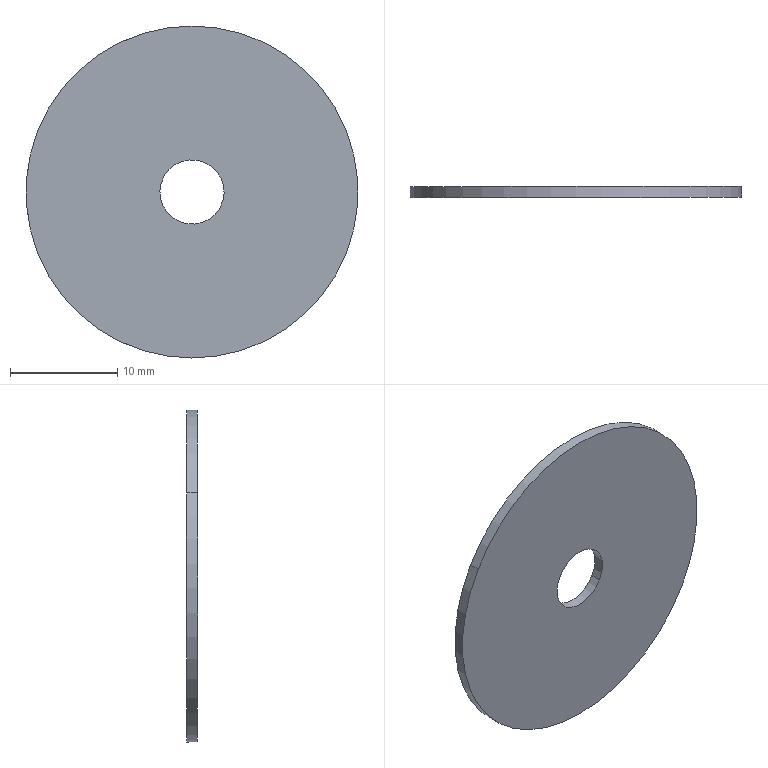Part | SolidWorks | features BaseBody 1 | 1 solid | 6 faces | box 31.001 x 1.03 x 31 mm | volume 726.493 mm3 | cylinder 4 | plane 2 | commonest cylinder face diameters 6 x2 31 x2
STEP:
#1=CARTESIAN_POINT('',(344.556,387.967,105.419));
#2=VERTEX_POINT('',#1);
#3=CARTESIAN_POINT('',(339.359,387.962,108.419));
#4=VERTEX_POINT('',#3);
#5=CARTESIAN_POINT('',(341.958,387.964,106.919));
#6=DIRECTION('',(-0.0009599,1.,0.));
#7=DIRECTION('',(-0.866,-0.0008313,0.5));
#8=AXIS2_PLACEMENT_3D('',#5,#6,#7);
#9=CIRCLE('',#8,3.);
#10=EDGE_CURVE('',#2,#4,#9,.T.);
#11=ORIENTED_EDGE('',*,*,#10,.F.);
#12=CARTESIAN_POINT('',(344.555,388.967,105.419));
#13=VERTEX_POINT('',#12);
#14=CARTESIAN_POINT('',(344.556,387.967,105.419));
#15=DIRECTION('',(-0.0009599,1.,0.));
#16=VECTOR('',#15,1000.);
#17=LINE('',#14,#16);
#18=EDGE_CURVE('',#2,#13,#17,.T.);
#19=ORIENTED_EDGE('',*,*,#18,.T.);
#20=CARTESIAN_POINT('',(339.359,388.962,108.419));
#21=VERTEX_POINT('',#20);
#22=CARTESIAN_POINT('',(341.957,388.964,106.919));
#23=DIRECTION('',(0.0009599,-1.,0.));
#24=DIRECTION('',(0.866,0.0008313,-0.5));
#25=AXIS2_PLACEMENT_3D('',#22,#23,#24);
#26=CIRCLE('',#25,3.);
#27=EDGE_CURVE('',#21,#13,#26,.T.);
#28=ORIENTED_EDGE('',*,*,#27,.F.);
#29=CARTESIAN_POINT('',(339.359,387.962,108.419));
#30=DIRECTION('',(-0.0009599,1.,0.));
#31=VECTOR('',#30,1000.);
#32=LINE('',#29,#31);
#33=EDGE_CURVE('',#4,#21,#32,.T.);
#34=ORIENTED_EDGE('',*,*,#33,.F.);
#35=EDGE_LOOP('',(#11,#19,#28,#34));
#36=FACE_OUTER_BOUND('',#35,.T.);
#37=CARTESIAN_POINT('',(341.958,387.964,106.919));
#38=DIRECTION('',(-0.0009599,1.,0.));
#39=DIRECTION('',(-0.866,-0.0008313,0.5));
#40=AXIS2_PLACEMENT_3D('',#37,#38,#39);
#41=CYLINDRICAL_SURFACE('',#40,3.);
#42=ADVANCED_FACE('',(#36),#41,.F.);
#43=CARTESIAN_POINT('',(355.381,387.977,99.169));
#44=VERTEX_POINT('',#43);
#45=CARTESIAN_POINT('',(328.534,387.951,114.669));
#46=VERTEX_POINT('',#45);
#47=CARTESIAN_POINT('',(341.958,387.964,106.919));
#48=DIRECTION('',(0.0009599,-1.,0.));
#49=DIRECTION('',(0.866,0.0008313,-0.5));
#50=AXIS2_PLACEMENT_3D('',#47,#48,#49);
#51=CIRCLE('',#50,15.5);
#52=EDGE_CURVE('',#44,#46,#51,.T.);
#53=ORIENTED_EDGE('',*,*,#52,.F.);
#54=CARTESIAN_POINT('',(355.38,388.977,99.169));
#55=VERTEX_POINT('',#54);
#56=CARTESIAN_POINT('',(355.381,387.977,99.169));
#57=DIRECTION('',(-0.0009599,1.,0.));
#58=VECTOR('',#57,1000.);
#59=LINE('',#56,#58);
#60=EDGE_CURVE('',#44,#55,#59,.T.);
#61=ORIENTED_EDGE('',*,*,#60,.T.);
#62=CARTESIAN_POINT('',(328.533,388.951,114.669));
#63=VERTEX_POINT('',#62);
#64=CARTESIAN_POINT('',(341.957,388.964,106.919));
#65=DIRECTION('',(-0.0009599,1.,0.));
#66=DIRECTION('',(0.866,0.0008313,-0.5));
#67=AXIS2_PLACEMENT_3D('',#64,#65,#66);
#68=CIRCLE('',#67,15.5);
#69=EDGE_CURVE('',#63,#55,#68,.T.);
#70=ORIENTED_EDGE('',*,*,#69,.F.);
#71=CARTESIAN_POINT('',(328.534,387.951,114.669));
#72=DIRECTION('',(-0.0009599,1.,0.));
#73=VECTOR('',#72,1000.);
#74=LINE('',#71,#73);
#75=EDGE_CURVE('',#46,#63,#74,.T.);
#76=ORIENTED_EDGE('',*,*,#75,.F.);
#77=EDGE_LOOP('',(#53,#61,#70,#76));
#78=FACE_OUTER_BOUND('',#77,.T.);
#79=CARTESIAN_POINT('',(341.958,387.964,106.919));
#80=DIRECTION('',(-0.0009599,1.,0.));
#81=DIRECTION('',(-0.866,-0.0008313,0.5));
#82=AXIS2_PLACEMENT_3D('',#79,#80,#81);
#83=CYLINDRICAL_SURFACE('',#82,15.5);
#84=ADVANCED_FACE('',(#78),#83,.T.);
#85=ORIENTED_EDGE('',*,*,#27,.T.);
#86=CARTESIAN_POINT('',(341.957,388.964,106.919));
#87=DIRECTION('',(0.0009599,-1.,0.));
#88=DIRECTION('',(0.866,0.0008313,-0.5));
#89=AXIS2_PLACEMENT_3D('',#86,#87,#88);
#90=CIRCLE('',#89,3.);
#91=EDGE_CURVE('',#13,#21,#90,.T.);
#92=ORIENTED_EDGE('',*,*,#91,.T.);
#93=EDGE_LOOP('',(#85,#92));
#94=FACE_BOUND('',#93,.T.);
#95=ORIENTED_EDGE('',*,*,#69,.T.);
#96=CARTESIAN_POINT('',(341.957,388.964,106.919));
#97=DIRECTION('',(-0.0009599,1.,0.));
#98=DIRECTION('',(0.866,0.0008313,-0.5));
#99=AXIS2_PLACEMENT_3D('',#96,#97,#98);
#100=CIRCLE('',#99,15.5);
#101=EDGE_CURVE('',#55,#63,#100,.T.);
#102=ORIENTED_EDGE('',*,*,#101,.T.);
#103=EDGE_LOOP('',(#95,#102));
#104=FACE_OUTER_BOUND('',#103,.T.);
#105=CARTESIAN_POINT('',(341.957,388.964,106.919));
#106=DIRECTION('',(0.0009599,-1.,0.));
#107=DIRECTION('',(0.,0.,-1.));
#108=AXIS2_PLACEMENT_3D('',#105,#106,#107);
#109=PLANE('',#108);
#110=ADVANCED_FACE('',(#94,#104),#109,.F.);
#111=ORIENTED_EDGE('',*,*,#60,.F.);
#112=CARTESIAN_POINT('',(341.958,387.964,106.919));
#113=DIRECTION('',(0.0009599,-1.,0.));
#114=DIRECTION('',(0.866,0.0008313,-0.5));
#115=AXIS2_PLACEMENT_3D('',#112,#113,#114);
#116=CIRCLE('',#115,15.5);
#117=EDGE_CURVE('',#46,#44,#116,.T.);
#118=ORIENTED_EDGE('',*,*,#117,.F.);
#119=ORIENTED_EDGE('',*,*,#75,.T.);
#120=ORIENTED_EDGE('',*,*,#101,.F.);
#121=EDGE_LOOP('',(#111,#118,#119,#120));
#122=FACE_OUTER_BOUND('',#121,.T.);
#123=CARTESIAN_POINT('',(341.958,387.964,106.919));
#124=DIRECTION('',(-0.0009599,1.,0.));
#125=DIRECTION('',(-0.866,-0.0008313,0.5));
#126=AXIS2_PLACEMENT_3D('',#123,#124,#125);
#127=CYLINDRICAL_SURFACE('',#126,15.5);
#128=ADVANCED_FACE('',(#122),#127,.T.);
#129=CARTESIAN_POINT('',(341.958,387.964,106.919));
#130=DIRECTION('',(-0.0009599,1.,0.));
#131=DIRECTION('',(-0.866,-0.0008313,0.5));
#132=AXIS2_PLACEMENT_3D('',#129,#130,#131);
#133=CIRCLE('',#132,3.);
#134=EDGE_CURVE('',#4,#2,#133,.T.);
#135=ORIENTED_EDGE('',*,*,#134,.T.);
#136=ORIENTED_EDGE('',*,*,#10,.T.);
#137=EDGE_LOOP('',(#135,#136));
#138=FACE_BOUND('',#137,.T.);
#139=ORIENTED_EDGE('',*,*,#117,.T.);
#140=ORIENTED_EDGE('',*,*,#52,.T.);
#141=EDGE_LOOP('',(#139,#140));
#142=FACE_OUTER_BOUND('',#141,.T.);
#143=CARTESIAN_POINT('',(341.958,387.964,106.919));
#144=DIRECTION('',(0.0009599,-1.,0.));
#145=DIRECTION('',(0.,0.,-1.));
#146=AXIS2_PLACEMENT_3D('',#143,#144,#145);
#147=PLANE('',#146);
#148=ADVANCED_FACE('',(#138,#142),#147,.T.);
#149=ORIENTED_EDGE('',*,*,#18,.F.);
#150=ORIENTED_EDGE('',*,*,#134,.F.);
#151=ORIENTED_EDGE('',*,*,#33,.T.);
#152=ORIENTED_EDGE('',*,*,#91,.F.);
#153=EDGE_LOOP('',(#149,#150,#151,#152));
#154=FACE_OUTER_BOUND('',#153,.T.);
#155=CARTESIAN_POINT('',(341.958,387.964,106.919));
#156=DIRECTION('',(-0.0009599,1.,0.));
#157=DIRECTION('',(-0.866,-0.0008313,0.5));
#158=AXIS2_PLACEMENT_3D('',#155,#156,#157);
#159=CYLINDRICAL_SURFACE('',#158,3.);
#160=ADVANCED_FACE('',(#154),#159,.F.);
#161=CLOSED_SHELL('',(#42,#84,#110,#128,#148,#160));
#162=MANIFOLD_SOLID_BREP('',#161);
#163=CARTESIAN_POINT('',(0.,0.,0.));
#164=DIRECTION('',(0.,0.,1.));
#165=DIRECTION('',(1.,0.,0.));
#166=AXIS2_PLACEMENT_3D('',#163,#164,#165);
#167=(LENGTH_UNIT()NAMED_UNIT(*)SI_UNIT(.MILLI.,.METRE.));
#168=UNCERTAINTY_MEASURE_WITH_UNIT(LENGTH_MEASURE(0.00001),#167,'','');
#169=(NAMED_UNIT(*)PLANE_ANGLE_UNIT()SI_UNIT($,.RADIAN.));
#170=(NAMED_UNIT(*)SI_UNIT($,.STERADIAN.)SOLID_ANGLE_UNIT());
#171=(GEOMETRIC_REPRESENTATION_CONTEXT(3)GLOBAL_UNCERTAINTY_ASSIGNED_CONTEXT((#168))GLOBAL_UNIT_ASSIGNED_CONTEXT((#167,#169,#170))REPRESENTATION_CONTEXT('',''));
#172=ADVANCED_BREP_SHAPE_REPRESENTATION('',(#162,#166),#171);